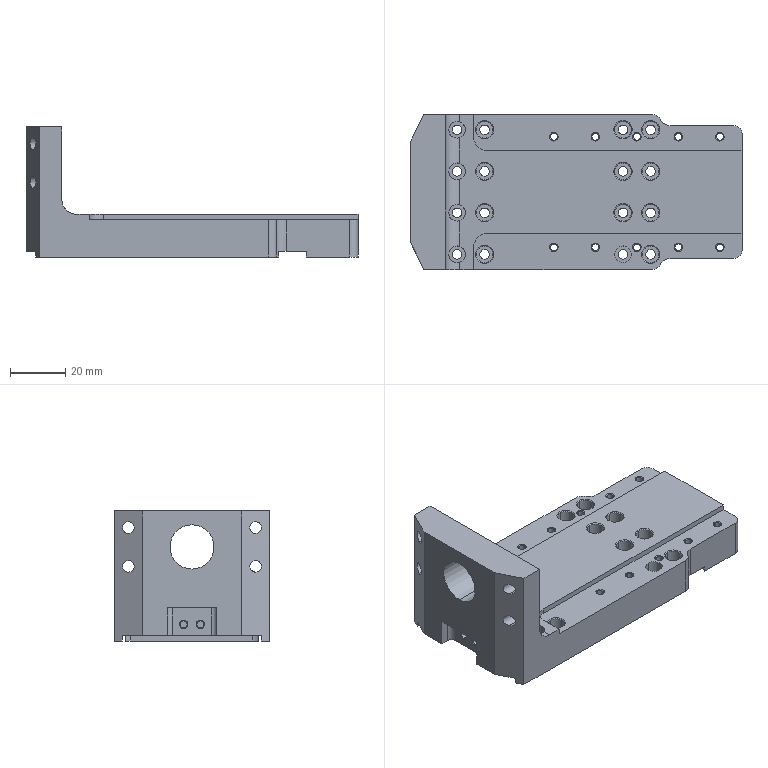Part | 1 solid | 272 faces | box 120 x 56 x 47 mm | volume 97166 mm3 | cylinder 117 | cone 106 | plane 49 | commonest cylinder face diameters 3.5 x32 5.999 x32 2.5 x24 4.2 x8 3.3 x6 6 x6